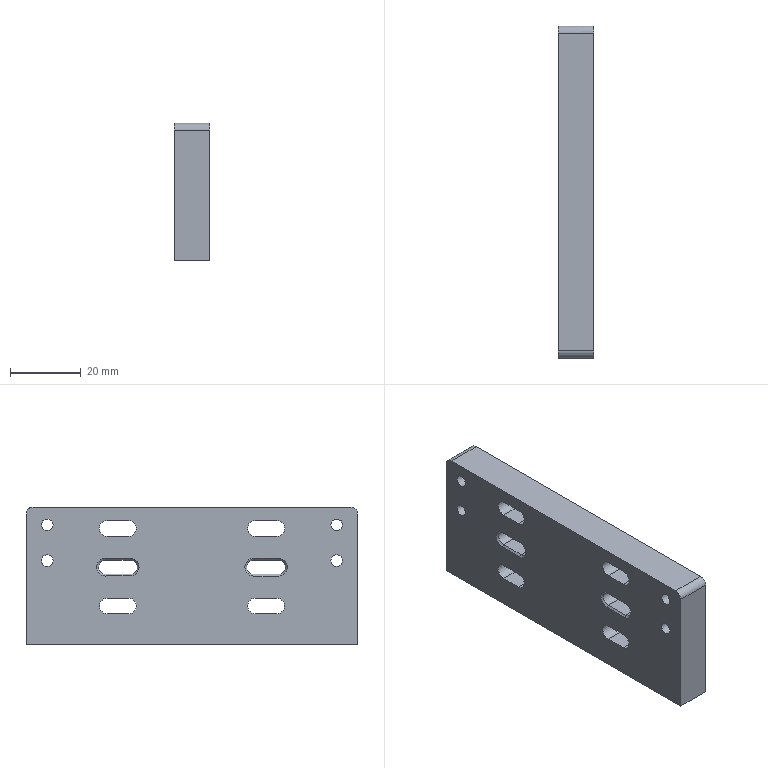Part | 1 solid | 88 faces | box 10.067 x 94 x 39 mm | volume 32633 mm3 | plane 46 | cylinder 26 | cone 16 | commonest cylinder face diameters 4.5 x8 8 x8 4 x6 3.3 x4